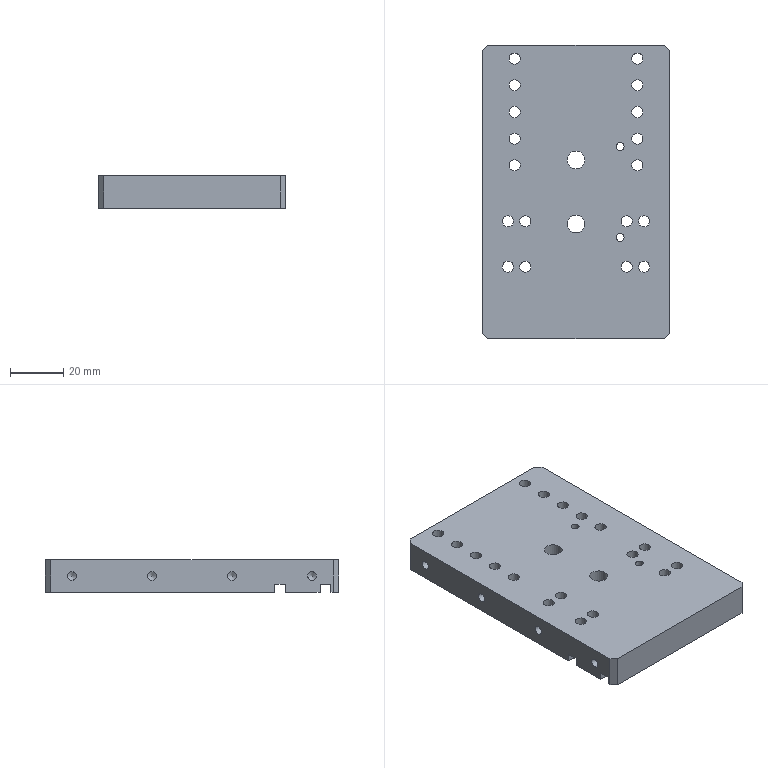CAM job | NX | 3-axis milling, drilling | part box 70 x 110 x 12 mm | stock box 75 x 115 x 15 mm
Tools:
number,name,description,diameter,corner_radius,flute_length,length,flutes
3,D3,平底铣刀-粗,3.0,0.0,20.0,75.0,2
6,D6,平底铣刀-粗,6.0,0.0,25.0,75.0,2
9,D10,平底铣刀-粗,10.0,0.0,35.0,75.0,2
11,D3-J,平底铣刀-精,3.0,0.0,50.0,75.0,2
7,D6-J,平底铣刀-精,6.0,0.0,25.0,75.0,2
1,D80R0.8飞刀,圆鼻刀-粗,80.0,0.8,50.0,75.0,2
1,D80R0.8飞刀-J,圆鼻刀-精,80.0,0.8,50.0,75.0,2
2,D6倒角刀,倒角刀,6.0,0.0,3.0,25.0,2
22,M5X0.8,丝锥,4.2,0.0,35.0,50.0,2
19,D3铰刀,Drilling Tool,3.0,0.0,75.0,100.0,6
18,钻头6.6,Drilling Tool,6.6,0.0,35.0,50.0,2
17,ZT2.9,Drilling Tool,2.9,0.0,35.0,50.0,2
14,ZT4.3,Drilling Tool,4.3,0.0,50.0,75.0,4
Operations:
program,operation,operation_type,tool,method,geometry_group,spindle_rpm,surface_speed,feed_per_tooth,feed_cut,feed_plunge,cut_length_mm,path_length_mm,cut_time_min,machine_time_min
B,底壁铣飞面开粗_COPY,VolumeBased25DMillingOperation,D80R0.8飞刀,分层开粗-切深K-步距G,W-B,2800.0,703.696,0.5357,3000.0,100.0,2084.614,2237.858,0.6949,0.7102
B,底壁铣飞面精光_COPY,VolumeBased25DMillingOperation,D80R0.8飞刀-J,侧刃精光-切深K-步距G,W-B,4000.0,1005.28,0.125,1000.0,100.0,416.373,512.373,0.4164,0.426
B,NG_钻倒角_2,Operation,D6倒角刀,METHOD,W-B,8000.0,150.796,0.0625,1000.0,0.0,9.6,156.332,0.0096,0.0243
B,NG_钻倒角_3,Operation,D6倒角刀,METHOD,W-B,8000.0,150.796,0.0625,1000.0,0.0,102.6,584.176,0.1026,0.1508
B,铣倒角_3,PlanarMilling,D6倒角刀,METHOD,W-B,8000.0,150.796,0.075,1200.0,100.0,40.892,266.317,0.0341,0.0566
B,平面去毛刺6X45L_COPY,SurfaceContour,D6倒角刀,爬面_倒角-切深0-步距G,W-B,6500.0,122.519,0.1154,1500.0,100.0,611.928,1231.352,0.408,0.4699
A,顶面,FaceMilling,D80R0.8飞刀,侧刃精光-切深K-步距G,W-A,4500.0,1385.0,0.1667,1500.0,100.0,444.0,540.0,0.296,0.3056
A,外形粗_2,VolumeBased25DMillingOperation,D10,METHOD,W-A,8000.0,251.327,0.375,6000.0,80.0,6586.598,6697.098,1.098,1.109
A,打点-深0.8,Operation,D6倒角刀,NONE,W-A,8000.0,150.796,0.0312,500.0,90.0,39.6,474.608,0.0792,0.1227
A,通孔-精孔3.0预钻,Operation,ZT2.9,NONE,W-A,3200.0,29.154,0.0312,200.0,90.0,33.674,202.363,0.1684,0.1852
A,通孔-M5螺纹底孔,Operation,ZT4.3,NONE,W-A,3000.0,39.584,0.0583,350.0,90.0,360.0,1058.579,1.029,1.098
A,沉头孔-钻孔0段,Operation,钻头6.6,NONE,W-A,1200.0,24.881,0.0625,150.0,90.0,33.81,192.642,0.2254,0.2413
A,底壁粗_1,VolumeBased25DMillingOperation,D3,METHOD,W-A,12000.0,113.097,0.0417,1000.0,100.0,4458.0,5018.082,4.458,4.514
A,铣孔开粗D6_1,CylinderMilling,D6,NONE,W-A,8000.0,150.796,0.075,1200.0,100.0,461.666,697.466,0.3847,0.4083
A,铣孔精光D6_1,CylinderMilling,D6-J,精光步距切深关,W-A,8000.0,150.796,0.0312,500.0,100.0,89.231,326.031,0.1785,0.2021
A,仅选体,SurfaceContour,D6倒角刀,METHOD,W-A,8000.0,150.796,0.1875,3000.0,100.0,672.266,1033.101,0.2241,0.2602
A,NG_钻倒角_1,Operation,D6倒角刀,METHOD,W-A,8000.0,150.796,0.0312,500.0,0.0,9.6,156.332,0.0192,0.0339
A,铣倒角_1,PlanarMilling,D6倒角刀,METHOD,W-A,8000.0,150.796,0.0312,500.0,100.0,324.366,2363.736,0.6487,0.8527
A,铣倒角_2,PlanarMilling,D6倒角刀,NONE,W-A,8000.0,150.796,0.05,800.0,100.0,86.785,299.096,0.1085,0.1297
A,REAMING,Operation,D3铰刀,METHOD,W-A,500.0,4.712,0.0167,50.0,0.0,28.0,191.015,0.56,0.5763
A,通孔-攻牙M5,Operation,M5X0.8,METHOD,W-A,500.0,6.597,0.0008,0.8,90.0,297.0,932.579,371.25,371.314
A,底侧精_3,VolumeBased25DMillingOperation,D3-J,METHOD,W-A,8000.0,75.398,0.05,800.0,100.0,308.846,536.766,0.3861,0.4088
A,外形半精_2,VolumeBased25DMillingOperation,D6-J,METHOD,W-A,9000.0,169.646,0.0667,1200.0,100.0,379.079,502.079,0.3159,0.3282